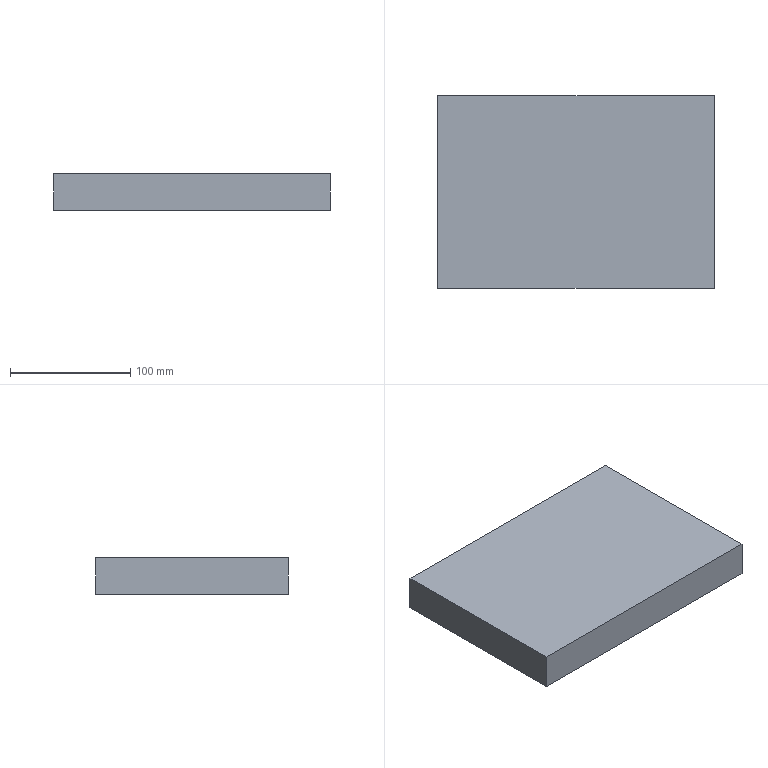Part | SolidWorks | features Extrusion 1 | 1 solid | 6 faces | box 230 x 160 x 30 mm | volume 1104000 mm3 | plane 6
STEP:
#1=CARTESIAN_POINT('',(0.,160.,0.));
#2=VERTEX_POINT('',#1);
#3=CARTESIAN_POINT('',(0.,0.,0.));
#4=VERTEX_POINT('',#3);
#5=CARTESIAN_POINT('',(0.,0.,0.));
#6=DIRECTION('',(0.,-1.,0.));
#7=VECTOR('',#6,1000.);
#8=LINE('',#5,#7);
#9=EDGE_CURVE('',#2,#4,#8,.T.);
#10=ORIENTED_EDGE('',*,*,#9,.T.);
#11=CARTESIAN_POINT('',(0.,0.,30.));
#12=VERTEX_POINT('',#11);
#13=CARTESIAN_POINT('',(0.,0.,30.));
#14=DIRECTION('',(0.,0.,-1.));
#15=VECTOR('',#14,1000.);
#16=LINE('',#13,#15);
#17=EDGE_CURVE('',#12,#4,#16,.T.);
#18=ORIENTED_EDGE('',*,*,#17,.F.);
#19=CARTESIAN_POINT('',(0.,160.,30.));
#20=VERTEX_POINT('',#19);
#21=CARTESIAN_POINT('',(0.,0.,30.));
#22=DIRECTION('',(0.,-1.,0.));
#23=VECTOR('',#22,1000.);
#24=LINE('',#21,#23);
#25=EDGE_CURVE('',#20,#12,#24,.T.);
#26=ORIENTED_EDGE('',*,*,#25,.F.);
#27=CARTESIAN_POINT('',(0.,160.,30.));
#28=DIRECTION('',(0.,0.,-1.));
#29=VECTOR('',#28,1000.);
#30=LINE('',#27,#29);
#31=EDGE_CURVE('',#20,#2,#30,.T.);
#32=ORIENTED_EDGE('',*,*,#31,.T.);
#33=EDGE_LOOP('',(#10,#18,#26,#32));
#34=FACE_OUTER_BOUND('',#33,.T.);
#35=CARTESIAN_POINT('',(0.,0.,30.));
#36=DIRECTION('',(1.,0.,0.));
#37=DIRECTION('',(0.,1.,0.));
#38=AXIS2_PLACEMENT_3D('',#35,#36,#37);
#39=PLANE('',#38);
#40=ADVANCED_FACE('',(#34),#39,.F.);
#41=CARTESIAN_POINT('',(230.,0.,0.));
#42=VERTEX_POINT('',#41);
#43=CARTESIAN_POINT('',(0.,0.,0.));
#44=DIRECTION('',(1.,0.,0.));
#45=VECTOR('',#44,1000.);
#46=LINE('',#43,#45);
#47=EDGE_CURVE('',#4,#42,#46,.T.);
#48=ORIENTED_EDGE('',*,*,#47,.T.);
#49=CARTESIAN_POINT('',(230.,0.,30.));
#50=VERTEX_POINT('',#49);
#51=CARTESIAN_POINT('',(230.,0.,30.));
#52=DIRECTION('',(0.,0.,-1.));
#53=VECTOR('',#52,1000.);
#54=LINE('',#51,#53);
#55=EDGE_CURVE('',#50,#42,#54,.T.);
#56=ORIENTED_EDGE('',*,*,#55,.F.);
#57=CARTESIAN_POINT('',(0.,0.,30.));
#58=DIRECTION('',(1.,0.,0.));
#59=VECTOR('',#58,1000.);
#60=LINE('',#57,#59);
#61=EDGE_CURVE('',#12,#50,#60,.T.);
#62=ORIENTED_EDGE('',*,*,#61,.F.);
#63=ORIENTED_EDGE('',*,*,#17,.T.);
#64=EDGE_LOOP('',(#48,#56,#62,#63));
#65=FACE_OUTER_BOUND('',#64,.T.);
#66=CARTESIAN_POINT('',(0.,0.,30.));
#67=DIRECTION('',(0.,1.,0.));
#68=DIRECTION('',(0.,0.,1.));
#69=AXIS2_PLACEMENT_3D('',#66,#67,#68);
#70=PLANE('',#69);
#71=ADVANCED_FACE('',(#65),#70,.F.);
#72=CARTESIAN_POINT('',(230.,160.,0.));
#73=VERTEX_POINT('',#72);
#74=CARTESIAN_POINT('',(230.,0.,0.));
#75=DIRECTION('',(0.,1.,0.));
#76=VECTOR('',#75,1000.);
#77=LINE('',#74,#76);
#78=EDGE_CURVE('',#42,#73,#77,.T.);
#79=ORIENTED_EDGE('',*,*,#78,.T.);
#80=CARTESIAN_POINT('',(230.,160.,30.));
#81=VERTEX_POINT('',#80);
#82=CARTESIAN_POINT('',(230.,160.,30.));
#83=DIRECTION('',(0.,0.,-1.));
#84=VECTOR('',#83,1000.);
#85=LINE('',#82,#84);
#86=EDGE_CURVE('',#81,#73,#85,.T.);
#87=ORIENTED_EDGE('',*,*,#86,.F.);
#88=CARTESIAN_POINT('',(230.,0.,30.));
#89=DIRECTION('',(0.,1.,0.));
#90=VECTOR('',#89,1000.);
#91=LINE('',#88,#90);
#92=EDGE_CURVE('',#50,#81,#91,.T.);
#93=ORIENTED_EDGE('',*,*,#92,.F.);
#94=ORIENTED_EDGE('',*,*,#55,.T.);
#95=EDGE_LOOP('',(#79,#87,#93,#94));
#96=FACE_OUTER_BOUND('',#95,.T.);
#97=CARTESIAN_POINT('',(230.,0.,30.));
#98=DIRECTION('',(-1.,0.,0.));
#99=DIRECTION('',(0.,-1.,0.));
#100=AXIS2_PLACEMENT_3D('',#97,#98,#99);
#101=PLANE('',#100);
#102=ADVANCED_FACE('',(#96),#101,.F.);
#103=CARTESIAN_POINT('',(0.,160.,0.));
#104=DIRECTION('',(-1.,0.,0.));
#105=VECTOR('',#104,1000.);
#106=LINE('',#103,#105);
#107=EDGE_CURVE('',#73,#2,#106,.T.);
#108=ORIENTED_EDGE('',*,*,#107,.T.);
#109=ORIENTED_EDGE('',*,*,#31,.F.);
#110=CARTESIAN_POINT('',(0.,160.,30.));
#111=DIRECTION('',(-1.,0.,0.));
#112=VECTOR('',#111,1000.);
#113=LINE('',#110,#112);
#114=EDGE_CURVE('',#81,#20,#113,.T.);
#115=ORIENTED_EDGE('',*,*,#114,.F.);
#116=ORIENTED_EDGE('',*,*,#86,.T.);
#117=EDGE_LOOP('',(#108,#109,#115,#116));
#118=FACE_OUTER_BOUND('',#117,.T.);
#119=CARTESIAN_POINT('',(0.,160.,30.));
#120=DIRECTION('',(0.,-1.,0.));
#121=DIRECTION('',(0.,0.,-1.));
#122=AXIS2_PLACEMENT_3D('',#119,#120,#121);
#123=PLANE('',#122);
#124=ADVANCED_FACE('',(#118),#123,.F.);
#125=ORIENTED_EDGE('',*,*,#25,.T.);
#126=ORIENTED_EDGE('',*,*,#61,.T.);
#127=ORIENTED_EDGE('',*,*,#92,.T.);
#128=ORIENTED_EDGE('',*,*,#114,.T.);
#129=EDGE_LOOP('',(#125,#126,#127,#128));
#130=FACE_OUTER_BOUND('',#129,.T.);
#131=CARTESIAN_POINT('',(0.,0.,30.));
#132=DIRECTION('',(0.,0.,-1.));
#133=DIRECTION('',(-1.,0.,0.));
#134=AXIS2_PLACEMENT_3D('',#131,#132,#133);
#135=PLANE('',#134);
#136=ADVANCED_FACE('',(#130),#135,.F.);
#137=ORIENTED_EDGE('',*,*,#9,.F.);
#138=ORIENTED_EDGE('',*,*,#107,.F.);
#139=ORIENTED_EDGE('',*,*,#78,.F.);
#140=ORIENTED_EDGE('',*,*,#47,.F.);
#141=EDGE_LOOP('',(#137,#138,#139,#140));
#142=FACE_OUTER_BOUND('',#141,.T.);
#143=CARTESIAN_POINT('',(0.,0.,0.));
#144=DIRECTION('',(0.,0.,-1.));
#145=DIRECTION('',(-1.,0.,0.));
#146=AXIS2_PLACEMENT_3D('',#143,#144,#145);
#147=PLANE('',#146);
#148=ADVANCED_FACE('',(#142),#147,.T.);
#149=CLOSED_SHELL('',(#40,#71,#102,#124,#136,#148));
#150=MANIFOLD_SOLID_BREP('',#149);
#151=CARTESIAN_POINT('',(0.,0.,0.));
#152=DIRECTION('',(0.,0.,1.));
#153=DIRECTION('',(1.,0.,0.));
#154=AXIS2_PLACEMENT_3D('',#151,#152,#153);
#155=(LENGTH_UNIT()NAMED_UNIT(*)SI_UNIT(.MILLI.,.METRE.));
#156=UNCERTAINTY_MEASURE_WITH_UNIT(LENGTH_MEASURE(0.00001),#155,'','');
#157=(NAMED_UNIT(*)PLANE_ANGLE_UNIT()SI_UNIT($,.RADIAN.));
#158=(NAMED_UNIT(*)SI_UNIT($,.STERADIAN.)SOLID_ANGLE_UNIT());
#159=(GEOMETRIC_REPRESENTATION_CONTEXT(3)GLOBAL_UNCERTAINTY_ASSIGNED_CONTEXT((#156))GLOBAL_UNIT_ASSIGNED_CONTEXT((#155,#157,#158))REPRESENTATION_CONTEXT('',''));
#160=ADVANCED_BREP_SHAPE_REPRESENTATION('',(#150,#154),#159);